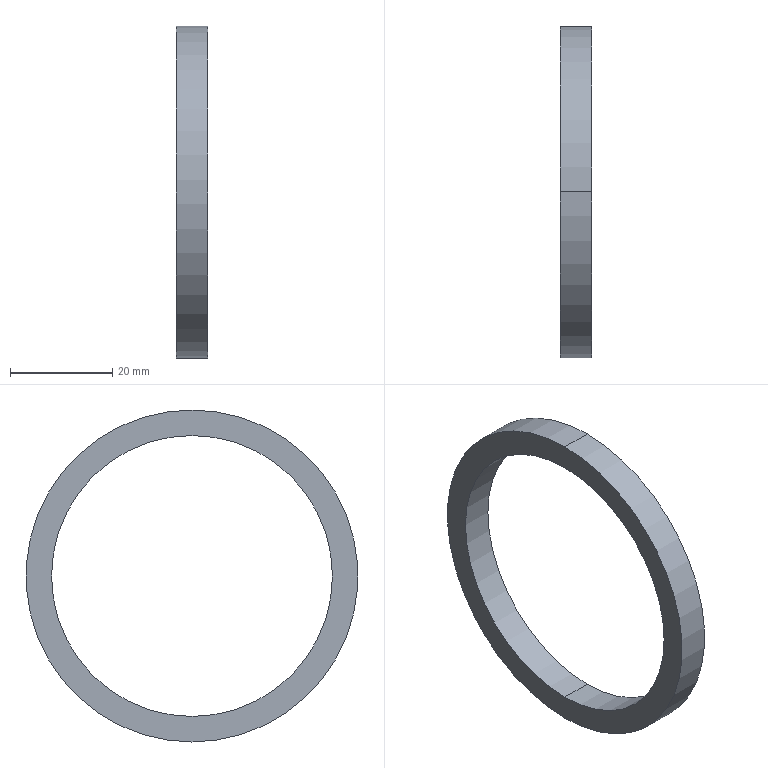Part | SolidWorks | features Extrusion 1 | 1 solid | 6 faces | box 6.2 x 65 x 65 mm | volume 5843 mm3 | cylinder 4 | plane 2 | commonest cylinder face diameters 55 x2 65 x2
STEP:
#1=CARTESIAN_POINT('',(6.2,0.,27.5));
#2=VERTEX_POINT('',#1);
#3=CARTESIAN_POINT('',(6.2,0.,-27.5));
#4=VERTEX_POINT('',#3);
#5=CARTESIAN_POINT('',(6.2,0.,0.));
#6=DIRECTION('',(1.,0.,0.));
#7=DIRECTION('',(0.,0.,-1.));
#8=AXIS2_PLACEMENT_3D('',#5,#6,#7);
#9=CIRCLE('',#8,27.5);
#10=EDGE_CURVE('',#2,#4,#9,.T.);
#11=ORIENTED_EDGE('',*,*,#10,.T.);
#12=CARTESIAN_POINT('',(0.,0.,-27.5));
#13=VERTEX_POINT('',#12);
#14=CARTESIAN_POINT('',(6.2,0.,-27.5));
#15=DIRECTION('',(-1.,0.,0.));
#16=VECTOR('',#15,1000.);
#17=LINE('',#14,#16);
#18=EDGE_CURVE('',#4,#13,#17,.T.);
#19=ORIENTED_EDGE('',*,*,#18,.T.);
#20=CARTESIAN_POINT('',(0.,0.,27.5));
#21=VERTEX_POINT('',#20);
#22=CARTESIAN_POINT('',(0.,0.,0.));
#23=DIRECTION('',(1.,0.,0.));
#24=DIRECTION('',(0.,0.,-1.));
#25=AXIS2_PLACEMENT_3D('',#22,#23,#24);
#26=CIRCLE('',#25,27.5);
#27=EDGE_CURVE('',#21,#13,#26,.T.);
#28=ORIENTED_EDGE('',*,*,#27,.F.);
#29=CARTESIAN_POINT('',(6.2,0.,27.5));
#30=DIRECTION('',(-1.,0.,0.));
#31=VECTOR('',#30,1000.);
#32=LINE('',#29,#31);
#33=EDGE_CURVE('',#2,#21,#32,.T.);
#34=ORIENTED_EDGE('',*,*,#33,.F.);
#35=EDGE_LOOP('',(#11,#19,#28,#34));
#36=FACE_OUTER_BOUND('',#35,.T.);
#37=CARTESIAN_POINT('',(6.2,0.,0.));
#38=DIRECTION('',(-1.,0.,0.));
#39=DIRECTION('',(0.,0.,1.));
#40=AXIS2_PLACEMENT_3D('',#37,#38,#39);
#41=CYLINDRICAL_SURFACE('',#40,27.5);
#42=ADVANCED_FACE('',(#36),#41,.F.);
#43=CARTESIAN_POINT('',(6.2,0.,-32.5));
#44=VERTEX_POINT('',#43);
#45=CARTESIAN_POINT('',(6.2,0.,32.5));
#46=VERTEX_POINT('',#45);
#47=CARTESIAN_POINT('',(6.2,0.,0.));
#48=DIRECTION('',(1.,0.,0.));
#49=DIRECTION('',(0.,0.,-1.));
#50=AXIS2_PLACEMENT_3D('',#47,#48,#49);
#51=CIRCLE('',#50,32.5);
#52=EDGE_CURVE('',#44,#46,#51,.T.);
#53=ORIENTED_EDGE('',*,*,#52,.F.);
#54=CARTESIAN_POINT('',(0.,0.,-32.5));
#55=VERTEX_POINT('',#54);
#56=CARTESIAN_POINT('',(6.2,0.,-32.5));
#57=DIRECTION('',(-1.,0.,0.));
#58=VECTOR('',#57,1000.);
#59=LINE('',#56,#58);
#60=EDGE_CURVE('',#44,#55,#59,.T.);
#61=ORIENTED_EDGE('',*,*,#60,.T.);
#62=CARTESIAN_POINT('',(0.,0.,32.5));
#63=VERTEX_POINT('',#62);
#64=CARTESIAN_POINT('',(0.,0.,0.));
#65=DIRECTION('',(1.,0.,0.));
#66=DIRECTION('',(0.,0.,-1.));
#67=AXIS2_PLACEMENT_3D('',#64,#65,#66);
#68=CIRCLE('',#67,32.5);
#69=EDGE_CURVE('',#55,#63,#68,.T.);
#70=ORIENTED_EDGE('',*,*,#69,.T.);
#71=CARTESIAN_POINT('',(6.2,0.,32.5));
#72=DIRECTION('',(-1.,0.,0.));
#73=VECTOR('',#72,1000.);
#74=LINE('',#71,#73);
#75=EDGE_CURVE('',#46,#63,#74,.T.);
#76=ORIENTED_EDGE('',*,*,#75,.F.);
#77=EDGE_LOOP('',(#53,#61,#70,#76));
#78=FACE_OUTER_BOUND('',#77,.T.);
#79=CARTESIAN_POINT('',(6.2,0.,0.));
#80=DIRECTION('',(-1.,0.,0.));
#81=DIRECTION('',(0.,0.,1.));
#82=AXIS2_PLACEMENT_3D('',#79,#80,#81);
#83=CYLINDRICAL_SURFACE('',#82,32.5);
#84=ADVANCED_FACE('',(#78),#83,.T.);
#85=CARTESIAN_POINT('',(6.2,0.,0.));
#86=DIRECTION('',(1.,0.,0.));
#87=DIRECTION('',(0.,0.,-1.));
#88=AXIS2_PLACEMENT_3D('',#85,#86,#87);
#89=CIRCLE('',#88,32.5);
#90=EDGE_CURVE('',#46,#44,#89,.T.);
#91=ORIENTED_EDGE('',*,*,#90,.T.);
#92=ORIENTED_EDGE('',*,*,#52,.T.);
#93=EDGE_LOOP('',(#91,#92));
#94=FACE_OUTER_BOUND('',#93,.T.);
#95=ORIENTED_EDGE('',*,*,#10,.F.);
#96=CARTESIAN_POINT('',(6.2,0.,0.));
#97=DIRECTION('',(1.,0.,0.));
#98=DIRECTION('',(0.,0.,-1.));
#99=AXIS2_PLACEMENT_3D('',#96,#97,#98);
#100=CIRCLE('',#99,27.5);
#101=EDGE_CURVE('',#4,#2,#100,.T.);
#102=ORIENTED_EDGE('',*,*,#101,.F.);
#103=EDGE_LOOP('',(#95,#102));
#104=FACE_BOUND('',#103,.T.);
#105=CARTESIAN_POINT('',(6.2,0.,0.));
#106=DIRECTION('',(1.,0.,0.));
#107=DIRECTION('',(0.,0.,-1.));
#108=AXIS2_PLACEMENT_3D('',#105,#106,#107);
#109=PLANE('',#108);
#110=ADVANCED_FACE('',(#94,#104),#109,.T.);
#111=CARTESIAN_POINT('',(0.,0.,0.));
#112=DIRECTION('',(1.,0.,0.));
#113=DIRECTION('',(0.,0.,-1.));
#114=AXIS2_PLACEMENT_3D('',#111,#112,#113);
#115=CIRCLE('',#114,32.5);
#116=EDGE_CURVE('',#63,#55,#115,.T.);
#117=ORIENTED_EDGE('',*,*,#116,.F.);
#118=ORIENTED_EDGE('',*,*,#69,.F.);
#119=EDGE_LOOP('',(#117,#118));
#120=FACE_OUTER_BOUND('',#119,.T.);
#121=ORIENTED_EDGE('',*,*,#27,.T.);
#122=CARTESIAN_POINT('',(0.,0.,0.));
#123=DIRECTION('',(1.,0.,0.));
#124=DIRECTION('',(0.,0.,-1.));
#125=AXIS2_PLACEMENT_3D('',#122,#123,#124);
#126=CIRCLE('',#125,27.5);
#127=EDGE_CURVE('',#13,#21,#126,.T.);
#128=ORIENTED_EDGE('',*,*,#127,.T.);
#129=EDGE_LOOP('',(#121,#128));
#130=FACE_BOUND('',#129,.T.);
#131=CARTESIAN_POINT('',(0.,0.,0.));
#132=DIRECTION('',(1.,0.,0.));
#133=DIRECTION('',(0.,0.,-1.));
#134=AXIS2_PLACEMENT_3D('',#131,#132,#133);
#135=PLANE('',#134);
#136=ADVANCED_FACE('',(#120,#130),#135,.F.);
#137=ORIENTED_EDGE('',*,*,#60,.F.);
#138=ORIENTED_EDGE('',*,*,#90,.F.);
#139=ORIENTED_EDGE('',*,*,#75,.T.);
#140=ORIENTED_EDGE('',*,*,#116,.T.);
#141=EDGE_LOOP('',(#137,#138,#139,#140));
#142=FACE_OUTER_BOUND('',#141,.T.);
#143=CARTESIAN_POINT('',(6.2,0.,0.));
#144=DIRECTION('',(-1.,0.,0.));
#145=DIRECTION('',(0.,0.,1.));
#146=AXIS2_PLACEMENT_3D('',#143,#144,#145);
#147=CYLINDRICAL_SURFACE('',#146,32.5);
#148=ADVANCED_FACE('',(#142),#147,.T.);
#149=ORIENTED_EDGE('',*,*,#18,.F.);
#150=ORIENTED_EDGE('',*,*,#101,.T.);
#151=ORIENTED_EDGE('',*,*,#33,.T.);
#152=ORIENTED_EDGE('',*,*,#127,.F.);
#153=EDGE_LOOP('',(#149,#150,#151,#152));
#154=FACE_OUTER_BOUND('',#153,.T.);
#155=CARTESIAN_POINT('',(6.2,0.,0.));
#156=DIRECTION('',(-1.,0.,0.));
#157=DIRECTION('',(0.,0.,1.));
#158=AXIS2_PLACEMENT_3D('',#155,#156,#157);
#159=CYLINDRICAL_SURFACE('',#158,27.5);
#160=ADVANCED_FACE('',(#154),#159,.F.);
#161=CLOSED_SHELL('',(#42,#84,#110,#136,#148,#160));
#162=MANIFOLD_SOLID_BREP('',#161);
#163=CARTESIAN_POINT('',(0.,0.,0.));
#164=DIRECTION('',(0.,0.,1.));
#165=DIRECTION('',(1.,0.,0.));
#166=AXIS2_PLACEMENT_3D('',#163,#164,#165);
#167=(LENGTH_UNIT()NAMED_UNIT(*)SI_UNIT(.MILLI.,.METRE.));
#168=UNCERTAINTY_MEASURE_WITH_UNIT(LENGTH_MEASURE(0.00001),#167,'','');
#169=(NAMED_UNIT(*)PLANE_ANGLE_UNIT()SI_UNIT($,.RADIAN.));
#170=(NAMED_UNIT(*)SI_UNIT($,.STERADIAN.)SOLID_ANGLE_UNIT());
#171=(GEOMETRIC_REPRESENTATION_CONTEXT(3)GLOBAL_UNCERTAINTY_ASSIGNED_CONTEXT((#168))GLOBAL_UNIT_ASSIGNED_CONTEXT((#167,#169,#170))REPRESENTATION_CONTEXT('',''));
#172=ADVANCED_BREP_SHAPE_REPRESENTATION('',(#162,#166),#171);